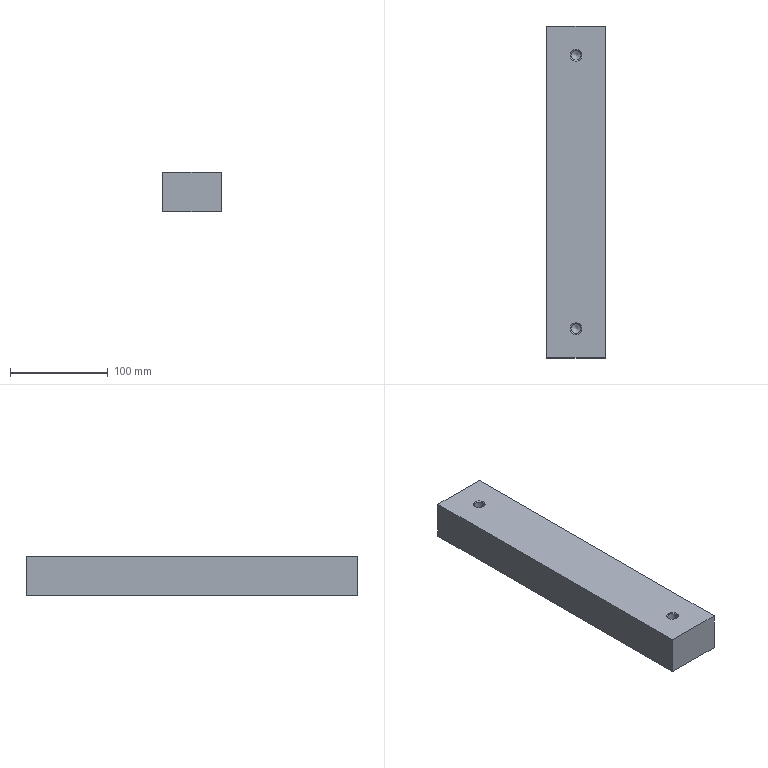Part | STEP file | 200 mesh_id2218 | 1 solid | 12 faces | box 60 x 340 x 40 mm | volume 809971 mm3 | plane 6 | cone 4 | cylinder 2 | commonest cylinder face diameters 10.3 x2
STEP:
#1=CARTESIAN_POINT('',(-16557.884,-4190.269,-90.));
#2=VERTEX_POINT('',#1);
#3=CARTESIAN_POINT('',(-16557.884,-3850.269,-90.));
#4=VERTEX_POINT('',#3);
#5=CARTESIAN_POINT('',(-16557.884,-4180.269,-90.));
#6=DIRECTION('',(0.,1.,0.));
#7=VECTOR('',#6,1.);
#8=LINE('',#5,#7);
#9=EDGE_CURVE('',#2,#4,#8,.T.);
#10=ORIENTED_EDGE('',*,*,#9,.T.);
#11=CARTESIAN_POINT('',(-16557.884,-3850.269,-50.));
#12=VERTEX_POINT('',#11);
#13=CARTESIAN_POINT('',(-16557.884,-3850.269,-50.));
#14=DIRECTION('',(0.,0.,-1.));
#15=VECTOR('',#14,1.);
#16=LINE('',#13,#15);
#17=EDGE_CURVE('',#12,#4,#16,.T.);
#18=ORIENTED_EDGE('',*,*,#17,.F.);
#19=CARTESIAN_POINT('',(-16557.884,-4190.269,-50.));
#20=VERTEX_POINT('',#19);
#21=CARTESIAN_POINT('',(-16557.884,-4180.269,-50.));
#22=DIRECTION('',(0.,1.,0.));
#23=VECTOR('',#22,1.);
#24=LINE('',#21,#23);
#25=EDGE_CURVE('',#20,#12,#24,.T.);
#26=ORIENTED_EDGE('',*,*,#25,.F.);
#27=CARTESIAN_POINT('',(-16557.884,-4190.269,-50.));
#28=DIRECTION('',(0.,0.,-1.));
#29=VECTOR('',#28,1.);
#30=LINE('',#27,#29);
#31=EDGE_CURVE('',#20,#2,#30,.T.);
#32=ORIENTED_EDGE('',*,*,#31,.T.);
#33=EDGE_LOOP('',(#10,#18,#26,#32));
#34=FACE_OUTER_BOUND('',#33,.T.);
#35=CARTESIAN_POINT('',(-16557.884,-4180.269,-50.));
#36=DIRECTION('',(-1.,0.,0.));
#37=DIRECTION('',(0.,0.,1.));
#38=AXIS2_PLACEMENT_3D('',#35,#36,#37);
#39=PLANE('',#38);
#40=ADVANCED_FACE('',(#34),#39,.F.);
#41=CARTESIAN_POINT('',(-16617.884,-3850.269,-90.));
#42=VERTEX_POINT('',#41);
#43=CARTESIAN_POINT('',(-16557.884,-3850.269,-90.));
#44=DIRECTION('',(-1.,0.,0.));
#45=VECTOR('',#44,1.);
#46=LINE('',#43,#45);
#47=EDGE_CURVE('',#4,#42,#46,.T.);
#48=ORIENTED_EDGE('',*,*,#47,.T.);
#49=CARTESIAN_POINT('',(-16617.884,-3850.269,-50.));
#50=VERTEX_POINT('',#49);
#51=CARTESIAN_POINT('',(-16617.884,-3850.269,-50.));
#52=DIRECTION('',(0.,0.,-1.));
#53=VECTOR('',#52,1.);
#54=LINE('',#51,#53);
#55=EDGE_CURVE('',#50,#42,#54,.T.);
#56=ORIENTED_EDGE('',*,*,#55,.F.);
#57=CARTESIAN_POINT('',(-16557.884,-3850.269,-50.));
#58=DIRECTION('',(-1.,0.,0.));
#59=VECTOR('',#58,1.);
#60=LINE('',#57,#59);
#61=EDGE_CURVE('',#12,#50,#60,.T.);
#62=ORIENTED_EDGE('',*,*,#61,.F.);
#63=ORIENTED_EDGE('',*,*,#17,.T.);
#64=EDGE_LOOP('',(#48,#56,#62,#63));
#65=FACE_OUTER_BOUND('',#64,.T.);
#66=CARTESIAN_POINT('',(-16557.884,-3850.269,-50.));
#67=DIRECTION('',(0.,-1.,0.));
#68=DIRECTION('',(0.,0.,-1.));
#69=AXIS2_PLACEMENT_3D('',#66,#67,#68);
#70=PLANE('',#69);
#71=ADVANCED_FACE('',(#65),#70,.F.);
#72=CARTESIAN_POINT('',(-16617.884,-4190.269,-90.));
#73=VERTEX_POINT('',#72);
#74=CARTESIAN_POINT('',(-16617.884,-3860.269,-90.));
#75=DIRECTION('',(0.,-1.,0.));
#76=VECTOR('',#75,1.);
#77=LINE('',#74,#76);
#78=EDGE_CURVE('',#42,#73,#77,.T.);
#79=ORIENTED_EDGE('',*,*,#78,.T.);
#80=CARTESIAN_POINT('',(-16617.884,-4190.269,-50.));
#81=VERTEX_POINT('',#80);
#82=CARTESIAN_POINT('',(-16617.884,-4190.269,-50.));
#83=DIRECTION('',(0.,0.,-1.));
#84=VECTOR('',#83,1.);
#85=LINE('',#82,#84);
#86=EDGE_CURVE('',#81,#73,#85,.T.);
#87=ORIENTED_EDGE('',*,*,#86,.F.);
#88=CARTESIAN_POINT('',(-16617.884,-3860.269,-50.));
#89=DIRECTION('',(0.,-1.,0.));
#90=VECTOR('',#89,1.);
#91=LINE('',#88,#90);
#92=EDGE_CURVE('',#50,#81,#91,.T.);
#93=ORIENTED_EDGE('',*,*,#92,.F.);
#94=ORIENTED_EDGE('',*,*,#55,.T.);
#95=EDGE_LOOP('',(#79,#87,#93,#94));
#96=FACE_OUTER_BOUND('',#95,.T.);
#97=CARTESIAN_POINT('',(-16617.884,-3860.269,-50.));
#98=DIRECTION('',(1.,0.,0.));
#99=DIRECTION('',(0.,0.,-1.));
#100=AXIS2_PLACEMENT_3D('',#97,#98,#99);
#101=PLANE('',#100);
#102=ADVANCED_FACE('',(#96),#101,.F.);
#103=CARTESIAN_POINT('',(-16617.884,-4190.269,-90.));
#104=DIRECTION('',(1.,0.,0.));
#105=VECTOR('',#104,1.);
#106=LINE('',#103,#105);
#107=EDGE_CURVE('',#73,#2,#106,.T.);
#108=ORIENTED_EDGE('',*,*,#107,.T.);
#109=ORIENTED_EDGE('',*,*,#31,.F.);
#110=CARTESIAN_POINT('',(-16617.884,-4190.269,-50.));
#111=DIRECTION('',(1.,0.,0.));
#112=VECTOR('',#111,1.);
#113=LINE('',#110,#112);
#114=EDGE_CURVE('',#81,#20,#113,.T.);
#115=ORIENTED_EDGE('',*,*,#114,.F.);
#116=ORIENTED_EDGE('',*,*,#86,.T.);
#117=EDGE_LOOP('',(#108,#109,#115,#116));
#118=FACE_OUTER_BOUND('',#117,.T.);
#119=CARTESIAN_POINT('',(-16617.884,-4190.269,-50.));
#120=DIRECTION('',(0.,1.,0.));
#121=DIRECTION('',(0.,0.,1.));
#122=AXIS2_PLACEMENT_3D('',#119,#120,#121);
#123=PLANE('',#122);
#124=ADVANCED_FACE('',(#118),#123,.F.);
#125=CARTESIAN_POINT('',(-16581.884,-3880.269,-50.));
#126=VERTEX_POINT('',#125);
#127=CARTESIAN_POINT('',(-16587.884,-3880.269,-50.));
#128=DIRECTION('',(0.,0.,-1.));
#129=DIRECTION('',(1.,0.,0.));
#130=AXIS2_PLACEMENT_3D('',#127,#128,#129);
#131=CIRCLE('',#130,6.);
#132=EDGE_CURVE('',#126,#126,#131,.T.);
#133=ORIENTED_EDGE('',*,*,#132,.T.);
#134=EDGE_LOOP('',(#133));
#135=FACE_BOUND('',#134,.T.);
#136=CARTESIAN_POINT('',(-16581.884,-4160.269,-50.));
#137=VERTEX_POINT('',#136);
#138=CARTESIAN_POINT('',(-16587.884,-4160.269,-50.));
#139=DIRECTION('',(0.,0.,-1.));
#140=DIRECTION('',(1.,0.,0.));
#141=AXIS2_PLACEMENT_3D('',#138,#139,#140);
#142=CIRCLE('',#141,6.);
#143=EDGE_CURVE('',#137,#137,#142,.T.);
#144=ORIENTED_EDGE('',*,*,#143,.T.);
#145=EDGE_LOOP('',(#144));
#146=FACE_BOUND('',#145,.T.);
#147=ORIENTED_EDGE('',*,*,#25,.T.);
#148=ORIENTED_EDGE('',*,*,#61,.T.);
#149=ORIENTED_EDGE('',*,*,#92,.T.);
#150=ORIENTED_EDGE('',*,*,#114,.T.);
#151=EDGE_LOOP('',(#147,#148,#149,#150));
#152=FACE_BOUND('',#151,.T.);
#153=CARTESIAN_POINT('',(445.,0.,-50.));
#154=DIRECTION('',(0.,0.,1.));
#155=DIRECTION('',(1.,0.,0.));
#156=AXIS2_PLACEMENT_3D('',#153,#154,#155);
#157=PLANE('',#156);
#158=ADVANCED_FACE('',(#135,#146,#152),#157,.T.);
#159=ORIENTED_EDGE('',*,*,#9,.F.);
#160=ORIENTED_EDGE('',*,*,#107,.F.);
#161=ORIENTED_EDGE('',*,*,#78,.F.);
#162=ORIENTED_EDGE('',*,*,#47,.F.);
#163=EDGE_LOOP('',(#159,#160,#161,#162));
#164=FACE_OUTER_BOUND('',#163,.T.);
#165=CARTESIAN_POINT('',(445.,0.,-90.));
#166=DIRECTION('',(0.,0.,1.));
#167=DIRECTION('',(1.,0.,0.));
#168=AXIS2_PLACEMENT_3D('',#165,#166,#167);
#169=PLANE('',#168);
#170=ADVANCED_FACE('',(#164),#169,.F.);
#171=CARTESIAN_POINT('',(-16593.034,-4160.269,-85.));
#172=VERTEX_POINT('',#171);
#173=CARTESIAN_POINT('',(-16587.884,-4160.269,-85.));
#174=DIRECTION('',(0.,0.,1.));
#175=DIRECTION('',(-1.,0.,0.));
#176=AXIS2_PLACEMENT_3D('',#173,#174,#175);
#177=CIRCLE('',#176,5.15);
#178=EDGE_CURVE('',#172,#172,#177,.T.);
#179=ORIENTED_EDGE('',*,*,#178,.T.);
#180=EDGE_LOOP('',(#179));
#181=FACE_BOUND('',#180,.T.);
#182=CARTESIAN_POINT('',(-16587.884,-4160.269,-88.094));
#183=VERTEX_POINT('',#182);
#184=VERTEX_LOOP('',#183);
#185=FACE_BOUND('',#184,.T.);
#186=CARTESIAN_POINT('',(-16587.884,-4160.269,-85.));
#187=DIRECTION('',(0.,0.,1.));
#188=DIRECTION('',(1.,0.,0.));
#189=AXIS2_PLACEMENT_3D('',#186,#187,#188);
#190=CONICAL_SURFACE('',#189,5.15,59.);
#191=ADVANCED_FACE('',(#181,#185),#190,.F.);
#192=CARTESIAN_POINT('',(-16582.734,-4160.269,-50.85));
#193=VERTEX_POINT('',#192);
#194=CARTESIAN_POINT('',(-16587.884,-4160.269,-50.85));
#195=DIRECTION('',(0.,0.,1.));
#196=DIRECTION('',(1.,0.,0.));
#197=AXIS2_PLACEMENT_3D('',#194,#195,#196);
#198=CIRCLE('',#197,5.15);
#199=EDGE_CURVE('',#193,#193,#198,.T.);
#200=ORIENTED_EDGE('',*,*,#199,.T.);
#201=EDGE_LOOP('',(#200));
#202=FACE_BOUND('',#201,.T.);
#203=ORIENTED_EDGE('',*,*,#178,.F.);
#204=EDGE_LOOP('',(#203));
#205=FACE_BOUND('',#204,.T.);
#206=CARTESIAN_POINT('',(-16587.884,-4160.269,-50.));
#207=DIRECTION('',(0.,0.,-1.));
#208=DIRECTION('',(-1.,0.,0.));
#209=AXIS2_PLACEMENT_3D('',#206,#207,#208);
#210=CYLINDRICAL_SURFACE('',#209,5.15);
#211=ADVANCED_FACE('',(#202,#205),#210,.F.);
#212=ORIENTED_EDGE('',*,*,#199,.F.);
#213=EDGE_LOOP('',(#212));
#214=FACE_BOUND('',#213,.T.);
#215=ORIENTED_EDGE('',*,*,#143,.F.);
#216=EDGE_LOOP('',(#215));
#217=FACE_BOUND('',#216,.T.);
#218=CARTESIAN_POINT('',(-16587.884,-4160.269,-50.));
#219=DIRECTION('',(0.,0.,1.));
#220=DIRECTION('',(1.,0.,0.));
#221=AXIS2_PLACEMENT_3D('',#218,#219,#220);
#222=CONICAL_SURFACE('',#221,6.,45.);
#223=ADVANCED_FACE('',(#214,#217),#222,.F.);
#224=CARTESIAN_POINT('',(-16593.034,-3880.269,-85.));
#225=VERTEX_POINT('',#224);
#226=CARTESIAN_POINT('',(-16587.884,-3880.269,-85.));
#227=DIRECTION('',(0.,0.,1.));
#228=DIRECTION('',(-1.,0.,0.));
#229=AXIS2_PLACEMENT_3D('',#226,#227,#228);
#230=CIRCLE('',#229,5.15);
#231=EDGE_CURVE('',#225,#225,#230,.T.);
#232=ORIENTED_EDGE('',*,*,#231,.T.);
#233=EDGE_LOOP('',(#232));
#234=FACE_BOUND('',#233,.T.);
#235=CARTESIAN_POINT('',(-16587.884,-3880.269,-88.094));
#236=VERTEX_POINT('',#235);
#237=VERTEX_LOOP('',#236);
#238=FACE_BOUND('',#237,.T.);
#239=CARTESIAN_POINT('',(-16587.884,-3880.269,-85.));
#240=DIRECTION('',(0.,0.,1.));
#241=DIRECTION('',(1.,0.,0.));
#242=AXIS2_PLACEMENT_3D('',#239,#240,#241);
#243=CONICAL_SURFACE('',#242,5.15,59.);
#244=ADVANCED_FACE('',(#234,#238),#243,.F.);
#245=CARTESIAN_POINT('',(-16582.734,-3880.269,-50.85));
#246=VERTEX_POINT('',#245);
#247=CARTESIAN_POINT('',(-16587.884,-3880.269,-50.85));
#248=DIRECTION('',(0.,0.,1.));
#249=DIRECTION('',(1.,0.,0.));
#250=AXIS2_PLACEMENT_3D('',#247,#248,#249);
#251=CIRCLE('',#250,5.15);
#252=EDGE_CURVE('',#246,#246,#251,.T.);
#253=ORIENTED_EDGE('',*,*,#252,.T.);
#254=EDGE_LOOP('',(#253));
#255=FACE_BOUND('',#254,.T.);
#256=ORIENTED_EDGE('',*,*,#231,.F.);
#257=EDGE_LOOP('',(#256));
#258=FACE_BOUND('',#257,.T.);
#259=CARTESIAN_POINT('',(-16587.884,-3880.269,-50.));
#260=DIRECTION('',(0.,0.,-1.));
#261=DIRECTION('',(-1.,0.,0.));
#262=AXIS2_PLACEMENT_3D('',#259,#260,#261);
#263=CYLINDRICAL_SURFACE('',#262,5.15);
#264=ADVANCED_FACE('',(#255,#258),#263,.F.);
#265=ORIENTED_EDGE('',*,*,#252,.F.);
#266=EDGE_LOOP('',(#265));
#267=FACE_BOUND('',#266,.T.);
#268=ORIENTED_EDGE('',*,*,#132,.F.);
#269=EDGE_LOOP('',(#268));
#270=FACE_BOUND('',#269,.T.);
#271=CARTESIAN_POINT('',(-16587.884,-3880.269,-50.));
#272=DIRECTION('',(0.,0.,1.));
#273=DIRECTION('',(1.,0.,0.));
#274=AXIS2_PLACEMENT_3D('',#271,#272,#273);
#275=CONICAL_SURFACE('',#274,6.,45.);
#276=ADVANCED_FACE('',(#267,#270),#275,.F.);
#277=CLOSED_SHELL('',(#40,#71,#102,#124,#158,#170,#191,#211,#223,#244,#264,#276));
#278=MANIFOLD_SOLID_BREP('',#277);
#279=(LENGTH_UNIT()NAMED_UNIT(*)SI_UNIT(.MILLI.,.METRE.));
#280=UNCERTAINTY_MEASURE_WITH_UNIT(LENGTH_MEASURE(0.00002),#279,'','');
#281=(NAMED_UNIT(*)PLANE_ANGLE_UNIT()SI_UNIT($,.RADIAN.));
#282=PLANE_ANGLE_MEASURE_WITH_UNIT(PLANE_ANGLE_MEASURE(0.01745),#281);
#283=DIMENSIONAL_EXPONENTS(0.,0.,0.,0.,0.,0.,0.);
#284=(CONVERSION_BASED_UNIT('DEGREE',#282)NAMED_UNIT(#283)PLANE_ANGLE_UNIT());
#285=(NAMED_UNIT(*)SI_UNIT($,.STERADIAN.)SOLID_ANGLE_UNIT());
#286=(GEOMETRIC_REPRESENTATION_CONTEXT(3)GLOBAL_UNCERTAINTY_ASSIGNED_CONTEXT((#280))GLOBAL_UNIT_ASSIGNED_CONTEXT((#279,#284,#285))REPRESENTATION_CONTEXT('',''));
#287=ADVANCED_BREP_SHAPE_REPRESENTATION('',(#278),#286);